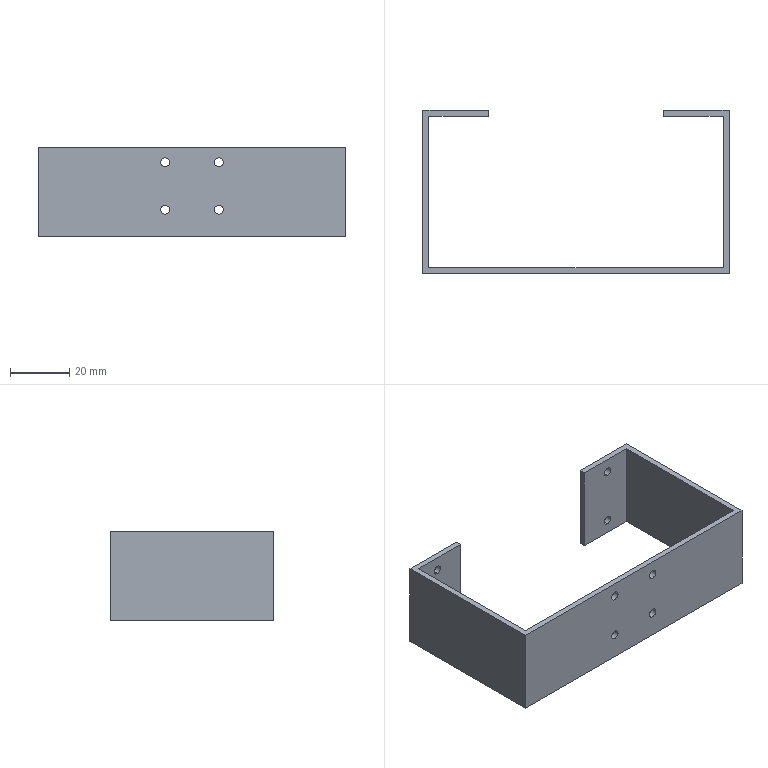Part | SolidWorks | features BaseBody 1 | 1 solid | 30 faces | box 103 x 55 x 30 mm | volume 14827 mm3 | cylinder 16 | plane 14 | commonest cylinder face diameters 3 x16
STEP:
#1=CARTESIAN_POINT('',(-11.413,0.,25.));
#2=VERTEX_POINT('',#1);
#3=CARTESIAN_POINT('',(-8.413,0.,25.));
#4=VERTEX_POINT('',#3);
#5=CARTESIAN_POINT('',(-9.913,0.,25.));
#6=DIRECTION('',(0.,-1.,0.));
#7=DIRECTION('',(1.,0.,0.));
#8=AXIS2_PLACEMENT_3D('',#5,#6,#7);
#9=CIRCLE('',#8,1.5);
#10=EDGE_CURVE('',#2,#4,#9,.T.);
#11=ORIENTED_EDGE('',*,*,#10,.F.);
#12=CARTESIAN_POINT('',(-11.413,-2.,25.));
#13=VERTEX_POINT('',#12);
#14=CARTESIAN_POINT('',(-11.413,8.,25.));
#15=DIRECTION('',(0.,-1.,0.));
#16=VECTOR('',#15,1000.);
#17=LINE('',#14,#16);
#18=EDGE_CURVE('',#2,#13,#17,.T.);
#19=ORIENTED_EDGE('',*,*,#18,.T.);
#20=CARTESIAN_POINT('',(-8.413,-2.,25.));
#21=VERTEX_POINT('',#20);
#22=CARTESIAN_POINT('',(-9.913,-2.,25.));
#23=DIRECTION('',(0.,1.,0.));
#24=DIRECTION('',(1.,0.,0.));
#25=AXIS2_PLACEMENT_3D('',#22,#23,#24);
#26=CIRCLE('',#25,1.5);
#27=EDGE_CURVE('',#21,#13,#26,.T.);
#28=ORIENTED_EDGE('',*,*,#27,.F.);
#29=CARTESIAN_POINT('',(-8.413,8.,25.));
#30=DIRECTION('',(0.,-1.,0.));
#31=VECTOR('',#30,1000.);
#32=LINE('',#29,#31);
#33=EDGE_CURVE('',#4,#21,#32,.T.);
#34=ORIENTED_EDGE('',*,*,#33,.F.);
#35=EDGE_LOOP('',(#11,#19,#28,#34));
#36=FACE_OUTER_BOUND('',#35,.T.);
#37=CARTESIAN_POINT('',(-9.913,8.,25.));
#38=DIRECTION('',(0.,-1.,0.));
#39=DIRECTION('',(1.,0.,0.));
#40=AXIS2_PLACEMENT_3D('',#37,#38,#39);
#41=CYLINDRICAL_SURFACE('',#40,1.5);
#42=ADVANCED_FACE('',(#36),#41,.F.);
#43=CARTESIAN_POINT('',(6.587,0.,9.));
#44=VERTEX_POINT('',#43);
#45=CARTESIAN_POINT('',(9.587,0.,9.));
#46=VERTEX_POINT('',#45);
#47=CARTESIAN_POINT('',(8.087,0.,9.));
#48=DIRECTION('',(0.,-1.,0.));
#49=DIRECTION('',(1.,0.,0.));
#50=AXIS2_PLACEMENT_3D('',#47,#48,#49);
#51=CIRCLE('',#50,1.5);
#52=EDGE_CURVE('',#44,#46,#51,.T.);
#53=ORIENTED_EDGE('',*,*,#52,.F.);
#54=CARTESIAN_POINT('',(6.587,-2.,9.));
#55=VERTEX_POINT('',#54);
#56=CARTESIAN_POINT('',(6.587,8.,9.));
#57=DIRECTION('',(0.,-1.,0.));
#58=VECTOR('',#57,1000.);
#59=LINE('',#56,#58);
#60=EDGE_CURVE('',#44,#55,#59,.T.);
#61=ORIENTED_EDGE('',*,*,#60,.T.);
#62=CARTESIAN_POINT('',(9.587,-2.,9.));
#63=VERTEX_POINT('',#62);
#64=CARTESIAN_POINT('',(8.087,-2.,9.));
#65=DIRECTION('',(0.,1.,0.));
#66=DIRECTION('',(1.,0.,0.));
#67=AXIS2_PLACEMENT_3D('',#64,#65,#66);
#68=CIRCLE('',#67,1.5);
#69=EDGE_CURVE('',#63,#55,#68,.T.);
#70=ORIENTED_EDGE('',*,*,#69,.F.);
#71=CARTESIAN_POINT('',(9.587,8.,9.));
#72=DIRECTION('',(0.,-1.,0.));
#73=VECTOR('',#72,1000.);
#74=LINE('',#71,#73);
#75=EDGE_CURVE('',#46,#63,#74,.T.);
#76=ORIENTED_EDGE('',*,*,#75,.F.);
#77=EDGE_LOOP('',(#53,#61,#70,#76));
#78=FACE_OUTER_BOUND('',#77,.T.);
#79=CARTESIAN_POINT('',(8.087,8.,9.));
#80=DIRECTION('',(0.,-1.,0.));
#81=DIRECTION('',(1.,0.,0.));
#82=AXIS2_PLACEMENT_3D('',#79,#80,#81);
#83=CYLINDRICAL_SURFACE('',#82,1.5);
#84=ADVANCED_FACE('',(#78),#83,.F.);
#85=CARTESIAN_POINT('',(-11.413,0.,9.));
#86=VERTEX_POINT('',#85);
#87=CARTESIAN_POINT('',(-8.413,0.,9.));
#88=VERTEX_POINT('',#87);
#89=CARTESIAN_POINT('',(-9.913,0.,9.));
#90=DIRECTION('',(0.,-1.,0.));
#91=DIRECTION('',(1.,0.,0.));
#92=AXIS2_PLACEMENT_3D('',#89,#90,#91);
#93=CIRCLE('',#92,1.5);
#94=EDGE_CURVE('',#86,#88,#93,.T.);
#95=ORIENTED_EDGE('',*,*,#94,.F.);
#96=CARTESIAN_POINT('',(-11.413,-2.,9.));
#97=VERTEX_POINT('',#96);
#98=CARTESIAN_POINT('',(-11.413,8.,9.));
#99=DIRECTION('',(0.,-1.,0.));
#100=VECTOR('',#99,1000.);
#101=LINE('',#98,#100);
#102=EDGE_CURVE('',#86,#97,#101,.T.);
#103=ORIENTED_EDGE('',*,*,#102,.T.);
#104=CARTESIAN_POINT('',(-8.413,-2.,9.));
#105=VERTEX_POINT('',#104);
#106=CARTESIAN_POINT('',(-9.913,-2.,9.));
#107=DIRECTION('',(0.,1.,0.));
#108=DIRECTION('',(1.,0.,0.));
#109=AXIS2_PLACEMENT_3D('',#106,#107,#108);
#110=CIRCLE('',#109,1.5);
#111=EDGE_CURVE('',#105,#97,#110,.T.);
#112=ORIENTED_EDGE('',*,*,#111,.F.);
#113=CARTESIAN_POINT('',(-8.413,8.,9.));
#114=DIRECTION('',(0.,-1.,0.));
#115=VECTOR('',#114,1000.);
#116=LINE('',#113,#115);
#117=EDGE_CURVE('',#88,#105,#116,.T.);
#118=ORIENTED_EDGE('',*,*,#117,.F.);
#119=EDGE_LOOP('',(#95,#103,#112,#118));
#120=FACE_OUTER_BOUND('',#119,.T.);
#121=CARTESIAN_POINT('',(-9.913,8.,9.));
#122=DIRECTION('',(0.,-1.,0.));
#123=DIRECTION('',(1.,0.,0.));
#124=AXIS2_PLACEMENT_3D('',#121,#122,#123);
#125=CYLINDRICAL_SURFACE('',#124,1.5);
#126=ADVANCED_FACE('',(#120),#125,.F.);
#127=CARTESIAN_POINT('',(6.587,0.,25.));
#128=VERTEX_POINT('',#127);
#129=CARTESIAN_POINT('',(9.587,0.,25.));
#130=VERTEX_POINT('',#129);
#131=CARTESIAN_POINT('',(8.087,0.,25.));
#132=DIRECTION('',(0.,-1.,0.));
#133=DIRECTION('',(1.,0.,0.));
#134=AXIS2_PLACEMENT_3D('',#131,#132,#133);
#135=CIRCLE('',#134,1.5);
#136=EDGE_CURVE('',#128,#130,#135,.T.);
#137=ORIENTED_EDGE('',*,*,#136,.F.);
#138=CARTESIAN_POINT('',(6.587,-2.,25.));
#139=VERTEX_POINT('',#138);
#140=CARTESIAN_POINT('',(6.587,8.,25.));
#141=DIRECTION('',(0.,-1.,0.));
#142=VECTOR('',#141,1000.);
#143=LINE('',#140,#142);
#144=EDGE_CURVE('',#128,#139,#143,.T.);
#145=ORIENTED_EDGE('',*,*,#144,.T.);
#146=CARTESIAN_POINT('',(9.587,-2.,25.));
#147=VERTEX_POINT('',#146);
#148=CARTESIAN_POINT('',(8.087,-2.,25.));
#149=DIRECTION('',(0.,1.,0.));
#150=DIRECTION('',(1.,0.,0.));
#151=AXIS2_PLACEMENT_3D('',#148,#149,#150);
#152=CIRCLE('',#151,1.5);
#153=EDGE_CURVE('',#147,#139,#152,.T.);
#154=ORIENTED_EDGE('',*,*,#153,.F.);
#155=CARTESIAN_POINT('',(9.587,8.,25.));
#156=DIRECTION('',(0.,-1.,0.));
#157=VECTOR('',#156,1000.);
#158=LINE('',#155,#157);
#159=EDGE_CURVE('',#130,#147,#158,.T.);
#160=ORIENTED_EDGE('',*,*,#159,.F.);
#161=EDGE_LOOP('',(#137,#145,#154,#160));
#162=FACE_OUTER_BOUND('',#161,.T.);
#163=CARTESIAN_POINT('',(8.087,8.,25.));
#164=DIRECTION('',(0.,-1.,0.));
#165=DIRECTION('',(1.,0.,0.));
#166=AXIS2_PLACEMENT_3D('',#163,#164,#165);
#167=CYLINDRICAL_SURFACE('',#166,1.5);
#168=ADVANCED_FACE('',(#162),#167,.F.);
#169=CARTESIAN_POINT('',(-41.413,51.,3.5));
#170=VERTEX_POINT('',#169);
#171=CARTESIAN_POINT('',(-41.413,51.,6.5));
#172=VERTEX_POINT('',#171);
#173=CARTESIAN_POINT('',(-41.413,51.,5.));
#174=DIRECTION('',(0.,1.,0.));
#175=DIRECTION('',(0.,0.,1.));
#176=AXIS2_PLACEMENT_3D('',#173,#174,#175);
#177=CIRCLE('',#176,1.5);
#178=EDGE_CURVE('',#170,#172,#177,.T.);
#179=ORIENTED_EDGE('',*,*,#178,.F.);
#180=CARTESIAN_POINT('',(-41.413,53.,3.5));
#181=VERTEX_POINT('',#180);
#182=CARTESIAN_POINT('',(-41.413,48.,3.5));
#183=DIRECTION('',(0.,1.,0.));
#184=VECTOR('',#183,1000.);
#185=LINE('',#182,#184);
#186=EDGE_CURVE('',#170,#181,#185,.T.);
#187=ORIENTED_EDGE('',*,*,#186,.T.);
#188=CARTESIAN_POINT('',(-41.413,53.,6.5));
#189=VERTEX_POINT('',#188);
#190=CARTESIAN_POINT('',(-41.413,53.,5.));
#191=DIRECTION('',(0.,-1.,0.));
#192=DIRECTION('',(0.,0.,1.));
#193=AXIS2_PLACEMENT_3D('',#190,#191,#192);
#194=CIRCLE('',#193,1.5);
#195=EDGE_CURVE('',#189,#181,#194,.T.);
#196=ORIENTED_EDGE('',*,*,#195,.F.);
#197=CARTESIAN_POINT('',(-41.413,48.,6.5));
#198=DIRECTION('',(0.,1.,0.));
#199=VECTOR('',#198,1000.);
#200=LINE('',#197,#199);
#201=EDGE_CURVE('',#172,#189,#200,.T.);
#202=ORIENTED_EDGE('',*,*,#201,.F.);
#203=EDGE_LOOP('',(#179,#187,#196,#202));
#204=FACE_OUTER_BOUND('',#203,.T.);
#205=CARTESIAN_POINT('',(-41.413,48.,5.));
#206=DIRECTION('',(0.,1.,0.));
#207=DIRECTION('',(0.,0.,1.));
#208=AXIS2_PLACEMENT_3D('',#205,#206,#207);
#209=CYLINDRICAL_SURFACE('',#208,1.5);
#210=ADVANCED_FACE('',(#204),#209,.F.);
#211=CARTESIAN_POINT('',(-41.413,51.,23.5));
#212=VERTEX_POINT('',#211);
#213=CARTESIAN_POINT('',(-41.413,51.,26.5));
#214=VERTEX_POINT('',#213);
#215=CARTESIAN_POINT('',(-41.413,51.,25.));
#216=DIRECTION('',(0.,1.,0.));
#217=DIRECTION('',(0.,0.,1.));
#218=AXIS2_PLACEMENT_3D('',#215,#216,#217);
#219=CIRCLE('',#218,1.5);
#220=EDGE_CURVE('',#212,#214,#219,.T.);
#221=ORIENTED_EDGE('',*,*,#220,.F.);
#222=CARTESIAN_POINT('',(-41.413,53.,23.5));
#223=VERTEX_POINT('',#222);
#224=CARTESIAN_POINT('',(-41.413,48.,23.5));
#225=DIRECTION('',(0.,1.,0.));
#226=VECTOR('',#225,1000.);
#227=LINE('',#224,#226);
#228=EDGE_CURVE('',#212,#223,#227,.T.);
#229=ORIENTED_EDGE('',*,*,#228,.T.);
#230=CARTESIAN_POINT('',(-41.413,53.,26.5));
#231=VERTEX_POINT('',#230);
#232=CARTESIAN_POINT('',(-41.413,53.,25.));
#233=DIRECTION('',(0.,-1.,0.));
#234=DIRECTION('',(0.,0.,1.));
#235=AXIS2_PLACEMENT_3D('',#232,#233,#234);
#236=CIRCLE('',#235,1.5);
#237=EDGE_CURVE('',#231,#223,#236,.T.);
#238=ORIENTED_EDGE('',*,*,#237,.F.);
#239=CARTESIAN_POINT('',(-41.413,48.,26.5));
#240=DIRECTION('',(0.,1.,0.));
#241=VECTOR('',#240,1000.);
#242=LINE('',#239,#241);
#243=EDGE_CURVE('',#214,#231,#242,.T.);
#244=ORIENTED_EDGE('',*,*,#243,.F.);
#245=EDGE_LOOP('',(#221,#229,#238,#244));
#246=FACE_OUTER_BOUND('',#245,.T.);
#247=CARTESIAN_POINT('',(-41.413,48.,25.));
#248=DIRECTION('',(0.,1.,0.));
#249=DIRECTION('',(0.,0.,1.));
#250=AXIS2_PLACEMENT_3D('',#247,#248,#249);
#251=CYLINDRICAL_SURFACE('',#250,1.5);
#252=ADVANCED_FACE('',(#246),#251,.F.);
#253=CARTESIAN_POINT('',(39.587,51.,26.5));
#254=VERTEX_POINT('',#253);
#255=CARTESIAN_POINT('',(39.587,51.,23.5));
#256=VERTEX_POINT('',#255);
#257=CARTESIAN_POINT('',(39.587,51.,25.));
#258=DIRECTION('',(0.,-1.,0.));
#259=DIRECTION('',(0.,0.,1.));
#260=AXIS2_PLACEMENT_3D('',#257,#258,#259);
#261=CIRCLE('',#260,1.5);
#262=EDGE_CURVE('',#254,#256,#261,.T.);
#263=ORIENTED_EDGE('',*,*,#262,.T.);
#264=CARTESIAN_POINT('',(39.587,53.,23.5));
#265=VERTEX_POINT('',#264);
#266=CARTESIAN_POINT('',(39.587,48.,23.5));
#267=DIRECTION('',(0.,1.,0.));
#268=VECTOR('',#267,1000.);
#269=LINE('',#266,#268);
#270=EDGE_CURVE('',#256,#265,#269,.T.);
#271=ORIENTED_EDGE('',*,*,#270,.T.);
#272=CARTESIAN_POINT('',(39.587,53.,26.5));
#273=VERTEX_POINT('',#272);
#274=CARTESIAN_POINT('',(39.587,53.,25.));
#275=DIRECTION('',(0.,1.,0.));
#276=DIRECTION('',(0.,0.,1.));
#277=AXIS2_PLACEMENT_3D('',#274,#275,#276);
#278=CIRCLE('',#277,1.5);
#279=EDGE_CURVE('',#265,#273,#278,.T.);
#280=ORIENTED_EDGE('',*,*,#279,.T.);
#281=CARTESIAN_POINT('',(39.587,48.,26.5));
#282=DIRECTION('',(0.,1.,0.));
#283=VECTOR('',#282,1000.);
#284=LINE('',#281,#283);
#285=EDGE_CURVE('',#254,#273,#284,.T.);
#286=ORIENTED_EDGE('',*,*,#285,.F.);
#287=EDGE_LOOP('',(#263,#271,#280,#286));
#288=FACE_OUTER_BOUND('',#287,.T.);
#289=CARTESIAN_POINT('',(39.587,48.,25.));
#290=DIRECTION('',(0.,1.,0.));
#291=DIRECTION('',(0.,0.,1.));
#292=AXIS2_PLACEMENT_3D('',#289,#290,#291);
#293=CYLINDRICAL_SURFACE('',#292,1.5);
#294=ADVANCED_FACE('',(#288),#293,.F.);
#295=CARTESIAN_POINT('',(39.587,51.,6.5));
#296=VERTEX_POINT('',#295);
#297=CARTESIAN_POINT('',(39.587,51.,3.5));
#298=VERTEX_POINT('',#297);
#299=CARTESIAN_POINT('',(39.587,51.,5.));
#300=DIRECTION('',(0.,-1.,0.));
#301=DIRECTION('',(0.,0.,1.));
#302=AXIS2_PLACEMENT_3D('',#299,#300,#301);
#303=CIRCLE('',#302,1.5);
#304=EDGE_CURVE('',#296,#298,#303,.T.);
#305=ORIENTED_EDGE('',*,*,#304,.T.);
#306=CARTESIAN_POINT('',(39.587,53.,3.5));
#307=VERTEX_POINT('',#306);
#308=CARTESIAN_POINT('',(39.587,48.,3.5));
#309=DIRECTION('',(0.,1.,0.));
#310=VECTOR('',#309,1000.);
#311=LINE('',#308,#310);
#312=EDGE_CURVE('',#298,#307,#311,.T.);
#313=ORIENTED_EDGE('',*,*,#312,.T.);
#314=CARTESIAN_POINT('',(39.587,53.,6.5));
#315=VERTEX_POINT('',#314);
#316=CARTESIAN_POINT('',(39.587,53.,5.));
#317=DIRECTION('',(0.,1.,0.));
#318=DIRECTION('',(0.,0.,1.));
#319=AXIS2_PLACEMENT_3D('',#316,#317,#318);
#320=CIRCLE('',#319,1.5);
#321=EDGE_CURVE('',#307,#315,#320,.T.);
#322=ORIENTED_EDGE('',*,*,#321,.T.);
#323=CARTESIAN_POINT('',(39.587,48.,6.5));
#324=DIRECTION('',(0.,1.,0.));
#325=VECTOR('',#324,1000.);
#326=LINE('',#323,#325);
#327=EDGE_CURVE('',#296,#315,#326,.T.);
#328=ORIENTED_EDGE('',*,*,#327,.F.);
#329=EDGE_LOOP('',(#305,#313,#322,#328));
#330=FACE_OUTER_BOUND('',#329,.T.);
#331=CARTESIAN_POINT('',(39.587,48.,5.));
#332=DIRECTION('',(0.,1.,0.));
#333=DIRECTION('',(0.,0.,1.));
#334=AXIS2_PLACEMENT_3D('',#331,#332,#333);
#335=CYLINDRICAL_SURFACE('',#334,1.5);
#336=ADVANCED_FACE('',(#330),#335,.F.);
#337=CARTESIAN_POINT('',(50.587,-2.,30.));
#338=VERTEX_POINT('',#337);
#339=CARTESIAN_POINT('',(-52.413,-2.,30.));
#340=VERTEX_POINT('',#339);
#341=CARTESIAN_POINT('',(0.,-2.,30.));
#342=DIRECTION('',(-1.,0.,0.));
#343=VECTOR('',#342,1000.);
#344=LINE('',#341,#343);
#345=EDGE_CURVE('',#338,#340,#344,.T.);
#346=ORIENTED_EDGE('',*,*,#345,.T.);
#347=CARTESIAN_POINT('',(-52.413,-2.,0.));
#348=VERTEX_POINT('',#347);
#349=CARTESIAN_POINT('',(-52.413,-2.,30.));
#350=DIRECTION('',(0.,0.,-1.));
#351=VECTOR('',#350,1000.);
#352=LINE('',#349,#351);
#353=EDGE_CURVE('',#340,#348,#352,.T.);
#354=ORIENTED_EDGE('',*,*,#353,.T.);
#355=CARTESIAN_POINT('',(50.587,-2.,0.));
#356=VERTEX_POINT('',#355);
#357=CARTESIAN_POINT('',(0.,-2.,0.));
#358=DIRECTION('',(1.,0.,0.));
#359=VECTOR('',#358,1000.);
#360=LINE('',#357,#359);
#361=EDGE_CURVE('',#348,#356,#360,.T.);
#362=ORIENTED_EDGE('',*,*,#361,.T.);
#363=CARTESIAN_POINT('',(50.587,-2.,30.));
#364=DIRECTION('',(0.,0.,1.));
#365=VECTOR('',#364,1000.);
#366=LINE('',#363,#365);
#367=EDGE_CURVE('',#356,#338,#366,.T.);
#368=ORIENTED_EDGE('',*,*,#367,.T.);
#369=EDGE_LOOP('',(#346,#354,#362,#368));
#370=FACE_OUTER_BOUND('',#369,.T.);
#371=ORIENTED_EDGE('',*,*,#27,.T.);
#372=CARTESIAN_POINT('',(-9.913,-2.,25.));
#373=DIRECTION('',(0.,1.,0.));
#374=DIRECTION('',(1.,0.,0.));
#375=AXIS2_PLACEMENT_3D('',#372,#373,#374);
#376=CIRCLE('',#375,1.5);
#377=EDGE_CURVE('',#13,#21,#376,.T.);
#378=ORIENTED_EDGE('',*,*,#377,.T.);
#379=EDGE_LOOP('',(#371,#378));
#380=FACE_BOUND('',#379,.T.);
#381=ORIENTED_EDGE('',*,*,#69,.T.);
#382=CARTESIAN_POINT('',(8.087,-2.,9.));
#383=DIRECTION('',(0.,1.,0.));
#384=DIRECTION('',(1.,0.,0.));
#385=AXIS2_PLACEMENT_3D('',#382,#383,#384);
#386=CIRCLE('',#385,1.5);
#387=EDGE_CURVE('',#55,#63,#386,.T.);
#388=ORIENTED_EDGE('',*,*,#387,.T.);
#389=EDGE_LOOP('',(#381,#388));
#390=FACE_BOUND('',#389,.T.);
#391=ORIENTED_EDGE('',*,*,#111,.T.);
#392=CARTESIAN_POINT('',(-9.913,-2.,9.));
#393=DIRECTION('',(0.,1.,0.));
#394=DIRECTION('',(1.,0.,0.));
#395=AXIS2_PLACEMENT_3D('',#392,#393,#394);
#396=CIRCLE('',#395,1.5);
#397=EDGE_CURVE('',#97,#105,#396,.T.);
#398=ORIENTED_EDGE('',*,*,#397,.T.);
#399=EDGE_LOOP('',(#391,#398));
#400=FACE_BOUND('',#399,.T.);
#401=ORIENTED_EDGE('',*,*,#153,.T.);
#402=CARTESIAN_POINT('',(8.087,-2.,25.));
#403=DIRECTION('',(0.,1.,0.));
#404=DIRECTION('',(1.,0.,0.));
#405=AXIS2_PLACEMENT_3D('',#402,#403,#404);
#406=CIRCLE('',#405,1.5);
#407=EDGE_CURVE('',#139,#147,#406,.T.);
#408=ORIENTED_EDGE('',*,*,#407,.T.);
#409=EDGE_LOOP('',(#401,#408));
#410=FACE_BOUND('',#409,.T.);
#411=CARTESIAN_POINT('',(0.,-2.,30.));
#412=DIRECTION('',(0.,-1.,0.));
#413=DIRECTION('',(1.,0.,0.));
#414=AXIS2_PLACEMENT_3D('',#411,#412,#413);
#415=PLANE('',#414);
#416=ADVANCED_FACE('',(#370,#380,#390,#400,#410),#415,.T.);
#417=CARTESIAN_POINT('',(-52.413,53.,30.));
#418=VERTEX_POINT('',#417);
#419=CARTESIAN_POINT('',(-52.413,0.,30.));
#420=DIRECTION('',(0.,1.,0.));
#421=VECTOR('',#420,1000.);
#422=LINE('',#419,#421);
#423=EDGE_CURVE('',#340,#418,#422,.T.);
#424=ORIENTED_EDGE('',*,*,#423,.T.);
#425=CARTESIAN_POINT('',(-52.413,53.,0.));
#426=VERTEX_POINT('',#425);
#427=CARTESIAN_POINT('',(-52.413,53.,30.));
#428=DIRECTION('',(0.,0.,-1.));
#429=VECTOR('',#428,1000.);
#430=LINE('',#427,#429);
#431=EDGE_CURVE('',#418,#426,#430,.T.);
#432=ORIENTED_EDGE('',*,*,#431,.T.);
#433=CARTESIAN_POINT('',(-52.413,0.,0.));
#434=DIRECTION('',(0.,-1.,0.));
#435=VECTOR('',#434,1000.);
#436=LINE('',#433,#435);
#437=EDGE_CURVE('',#426,#348,#436,.T.);
#438=ORIENTED_EDGE('',*,*,#437,.T.);
#439=ORIENTED_EDGE('',*,*,#353,.F.);
#440=EDGE_LOOP('',(#424,#432,#438,#439));
#441=FACE_OUTER_BOUND('',#440,.T.);
#442=CARTESIAN_POINT('',(-52.413,0.,30.));
#443=DIRECTION('',(-1.,0.,0.));
#444=DIRECTION('',(0.,0.,1.));
#445=AXIS2_PLACEMENT_3D('',#442,#443,#444);
#446=PLANE('',#445);
#447=ADVANCED_FACE('',(#441),#446,.T.);
#448=CARTESIAN_POINT('',(-30.413,53.,30.));
#449=VERTEX_POINT('',#448);
#450=CARTESIAN_POINT('',(0.,53.,30.));
#451=DIRECTION('',(-1.,0.,0.));
#452=VECTOR('',#451,1000.);
#453=LINE('',#450,#452);
#454=EDGE_CURVE('',#449,#418,#453,.T.);
#455=ORIENTED_EDGE('',*,*,#454,.T.);
#456=ORIENTED_EDGE('',*,*,#423,.F.);
#457=ORIENTED_EDGE('',*,*,#345,.F.);
#458=CARTESIAN_POINT('',(50.587,53.,30.));
#459=VERTEX_POINT('',#458);
#460=CARTESIAN_POINT('',(50.587,0.,30.));
#461=DIRECTION('',(0.,1.,0.));
#462=VECTOR('',#461,1000.);
#463=LINE('',#460,#462);
#464=EDGE_CURVE('',#338,#459,#463,.T.);
#465=ORIENTED_EDGE('',*,*,#464,.T.);
#466=CARTESIAN_POINT('',(28.587,53.,30.));
#467=VERTEX_POINT('',#466);
#468=CARTESIAN_POINT('',(0.,53.,30.));
#469=DIRECTION('',(-1.,0.,0.));
#470=VECTOR('',#469,1000.);
#471=LINE('',#468,#470);
#472=EDGE_CURVE('',#459,#467,#471,.T.);
#473=ORIENTED_EDGE('',*,*,#472,.T.);
#474=CARTESIAN_POINT('',(28.587,51.,30.));
#475=VERTEX_POINT('',#474);
#476=CARTESIAN_POINT('',(28.587,0.,30.));
#477=DIRECTION('',(0.,-1.,0.));
#478=VECTOR('',#477,1000.);
#479=LINE('',#476,#478);
#480=EDGE_CURVE('',#467,#475,#479,.T.);
#481=ORIENTED_EDGE('',*,*,#480,.T.);
#482=CARTESIAN_POINT('',(48.587,51.,30.));
#483=VERTEX_POINT('',#482);
#484=CARTESIAN_POINT('',(0.,51.,30.));
#485=DIRECTION('',(1.,0.,0.));
#486=VECTOR('',#485,1000.);
#487=LINE('',#484,#486);
#488=EDGE_CURVE('',#475,#483,#487,.T.);
#489=ORIENTED_EDGE('',*,*,#488,.T.);
#490=CARTESIAN_POINT('',(48.587,0.,30.));
#491=VERTEX_POINT('',#490);
#492=CARTESIAN_POINT('',(48.587,0.,30.));
#493=DIRECTION('',(0.,-1.,0.));
#494=VECTOR('',#493,1000.);
#495=LINE('',#492,#494);
#496=EDGE_CURVE('',#483,#491,#495,.T.);
#497=ORIENTED_EDGE('',*,*,#496,.T.);
#498=CARTESIAN_POINT('',(-50.413,0.,30.));
#499=VERTEX_POINT('',#498);
#500=CARTESIAN_POINT('',(0.,0.,30.));
#501=DIRECTION('',(-1.,0.,0.));
#502=VECTOR('',#501,1000.);
#503=LINE('',#500,#502);
#504=EDGE_CURVE('',#491,#499,#503,.T.);
#505=ORIENTED_EDGE('',*,*,#504,.T.);
#506=CARTESIAN_POINT('',(-50.413,51.,30.));
#507=VERTEX_POINT('',#506);
#508=CARTESIAN_POINT('',(-50.413,0.,30.));
#509=DIRECTION('',(0.,1.,0.));
#510=VECTOR('',#509,1000.);
#511=LINE('',#508,#510);
#512=EDGE_CURVE('',#499,#507,#511,.T.);
#513=ORIENTED_EDGE('',*,*,#512,.T.);
#514=CARTESIAN_POINT('',(-30.413,51.,30.));
#515=VERTEX_POINT('',#514);
#516=CARTESIAN_POINT('',(0.,51.,30.));
#517=DIRECTION('',(1.,0.,0.));
#518=VECTOR('',#517,1000.);
#519=LINE('',#516,#518);
#520=EDGE_CURVE('',#507,#515,#519,.T.);
#521=ORIENTED_EDGE('',*,*,#520,.T.);
#522=CARTESIAN_POINT('',(-30.413,0.,30.));
#523=DIRECTION('',(0.,1.,0.));
#524=VECTOR('',#523,1000.);
#525=LINE('',#522,#524);
#526=EDGE_CURVE('',#515,#449,#525,.T.);
#527=ORIENTED_EDGE('',*,*,#526,.T.);
#528=EDGE_LOOP('',(#455,#456,#457,#465,#473,#481,#489,#497,#505,#513,#521,#527));
#529=FACE_OUTER_BOUND('',#528,.T.);
#530=CARTESIAN_POINT('',(0.,0.,30.));
#531=DIRECTION('',(0.,0.,1.));
#532=DIRECTION('',(1.,0.,0.));
#533=AXIS2_PLACEMENT_3D('',#530,#531,#532);
#534=PLANE('',#533);
#535=ADVANCED_FACE('',(#529),#534,.T.);
#536=CARTESIAN_POINT('',(50.587,53.,0.));
#537=VERTEX_POINT('',#536);
#538=CARTESIAN_POINT('',(50.587,53.,30.));
#539=DIRECTION('',(0.,0.,-1.));
#540=VECTOR('',#539,1000.);
#541=LINE('',#538,#540);
#542=EDGE_CURVE('',#459,#537,#541,.T.);
#543=ORIENTED_EDGE('',*,*,#542,.F.);
#544=ORIENTED_EDGE('',*,*,#464,.F.);
#545=ORIENTED_EDGE('',*,*,#367,.F.);
#546=CARTESIAN_POINT('',(50.587,0.,0.));
#547=DIRECTION('',(0.,-1.,0.));
#548=VECTOR('',#547,1000.);
#549=LINE('',#546,#548);
#550=EDGE_CURVE('',#537,#356,#549,.T.);
#551=ORIENTED_EDGE('',*,*,#550,.F.);
#552=EDGE_LOOP('',(#543,#544,#545,#551));
#553=FACE_OUTER_BOUND('',#552,.T.);
#554=CARTESIAN_POINT('',(50.587,0.,30.));
#555=DIRECTION('',(-1.,0.,0.));
#556=DIRECTION('',(0.,-1.,0.));
#557=AXIS2_PLACEMENT_3D('',#554,#555,#556);
#558=PLANE('',#557);
#559=ADVANCED_FACE('',(#553),#558,.F.);
#560=ORIENTED_EDGE('',*,*,#437,.F.);
#561=CARTESIAN_POINT('',(-30.413,53.,0.));
#562=VERTEX_POINT('',#561);
#563=CARTESIAN_POINT('',(0.,53.,0.));
#564=DIRECTION('',(-1.,0.,0.));
#565=VECTOR('',#564,1000.);
#566=LINE('',#563,#565);
#567=EDGE_CURVE('',#562,#426,#566,.T.);
#568=ORIENTED_EDGE('',*,*,#567,.F.);
#569=CARTESIAN_POINT('',(-30.413,51.,0.));
#570=VERTEX_POINT('',#569);
#571=CARTESIAN_POINT('',(-30.413,0.,0.));
#572=DIRECTION('',(0.,1.,0.));
#573=VECTOR('',#572,1000.);
#574=LINE('',#571,#573);
#575=EDGE_CURVE('',#570,#562,#574,.T.);
#576=ORIENTED_EDGE('',*,*,#575,.F.);
#577=CARTESIAN_POINT('',(-50.413,51.,0.));
#578=VERTEX_POINT('',#577);
#579=CARTESIAN_POINT('',(0.,51.,0.));
#580=DIRECTION('',(1.,0.,0.));
#581=VECTOR('',#580,1000.);
#582=LINE('',#579,#581);
#583=EDGE_CURVE('',#578,#570,#582,.T.);
#584=ORIENTED_EDGE('',*,*,#583,.F.);
#585=CARTESIAN_POINT('',(-50.413,0.,0.));
#586=VERTEX_POINT('',#585);
#587=CARTESIAN_POINT('',(-50.413,0.,0.));
#588=DIRECTION('',(0.,1.,0.));
#589=VECTOR('',#588,1000.);
#590=LINE('',#587,#589);
#591=EDGE_CURVE('',#586,#578,#590,.T.);
#592=ORIENTED_EDGE('',*,*,#591,.F.);
#593=CARTESIAN_POINT('',(48.587,0.,0.));
#594=VERTEX_POINT('',#593);
#595=CARTESIAN_POINT('',(0.,0.,0.));
#596=DIRECTION('',(-1.,0.,0.));
#597=VECTOR('',#596,1000.);
#598=LINE('',#595,#597);
#599=EDGE_CURVE('',#594,#586,#598,.T.);
#600=ORIENTED_EDGE('',*,*,#599,.F.);
#601=CARTESIAN_POINT('',(48.587,51.,0.));
#602=VERTEX_POINT('',#601);
#603=CARTESIAN_POINT('',(48.587,0.,0.));
#604=DIRECTION('',(0.,-1.,0.));
#605=VECTOR('',#604,1000.);
#606=LINE('',#603,#605);
#607=EDGE_CURVE('',#602,#594,#606,.T.);
#608=ORIENTED_EDGE('',*,*,#607,.F.);
#609=CARTESIAN_POINT('',(28.587,51.,0.));
#610=VERTEX_POINT('',#609);
#611=CARTESIAN_POINT('',(0.,51.,0.));
#612=DIRECTION('',(1.,0.,0.));
#613=VECTOR('',#612,1000.);
#614=LINE('',#611,#613);
#615=EDGE_CURVE('',#610,#602,#614,.T.);
#616=ORIENTED_EDGE('',*,*,#615,.F.);
#617=CARTESIAN_POINT('',(28.587,53.,0.));
#618=VERTEX_POINT('',#617);
#619=CARTESIAN_POINT('',(28.587,0.,0.));
#620=DIRECTION('',(0.,-1.,0.));
#621=VECTOR('',#620,1000.);
#622=LINE('',#619,#621);
#623=EDGE_CURVE('',#618,#610,#622,.T.);
#624=ORIENTED_EDGE('',*,*,#623,.F.);
#625=CARTESIAN_POINT('',(0.,53.,0.));
#626=DIRECTION('',(-1.,0.,0.));
#627=VECTOR('',#626,1000.);
#628=LINE('',#625,#627);
#629=EDGE_CURVE('',#537,#618,#628,.T.);
#630=ORIENTED_EDGE('',*,*,#629,.F.);
#631=ORIENTED_EDGE('',*,*,#550,.T.);
#632=ORIENTED_EDGE('',*,*,#361,.F.);
#633=EDGE_LOOP('',(#560,#568,#576,#584,#592,#600,#608,#616,#624,#630,#631,#632));
#634=FACE_OUTER_BOUND('',#633,.T.);
#635=CARTESIAN_POINT('',(0.,0.,0.));
#636=DIRECTION('',(0.,0.,1.));
#637=DIRECTION('',(1.,0.,0.));
#638=AXIS2_PLACEMENT_3D('',#635,#636,#637);
#639=PLANE('',#638);
#640=ADVANCED_FACE('',(#634),#639,.F.);
#641=ORIENTED_EDGE('',*,*,#18,.F.);
#642=CARTESIAN_POINT('',(-9.913,0.,25.));
#643=DIRECTION('',(0.,-1.,0.));
#644=DIRECTION('',(1.,0.,0.));
#645=AXIS2_PLACEMENT_3D('',#642,#643,#644);
#646=CIRCLE('',#645,1.5);
#647=EDGE_CURVE('',#4,#2,#646,.T.);
#648=ORIENTED_EDGE('',*,*,#647,.F.);
#649=ORIENTED_EDGE('',*,*,#33,.T.);
#650=ORIENTED_EDGE('',*,*,#377,.F.);
#651=EDGE_LOOP('',(#641,#648,#649,#650));
#652=FACE_OUTER_BOUND('',#651,.T.);
#653=CARTESIAN_POINT('',(-9.913,8.,25.));
#654=DIRECTION('',(0.,-1.,0.));
#655=DIRECTION('',(1.,0.,0.));
#656=AXIS2_PLACEMENT_3D('',#653,#654,#655);
#657=CYLINDRICAL_SURFACE('',#656,1.5);
#658=ADVANCED_FACE('',(#652),#657,.F.);
#659=ORIENTED_EDGE('',*,*,#60,.F.);
#660=CARTESIAN_POINT('',(8.087,0.,9.));
#661=DIRECTION('',(0.,-1.,0.));
#662=DIRECTION('',(1.,0.,0.));
#663=AXIS2_PLACEMENT_3D('',#660,#661,#662);
#664=CIRCLE('',#663,1.5);
#665=EDGE_CURVE('',#46,#44,#664,.T.);
#666=ORIENTED_EDGE('',*,*,#665,.F.);
#667=ORIENTED_EDGE('',*,*,#75,.T.);
#668=ORIENTED_EDGE('',*,*,#387,.F.);
#669=EDGE_LOOP('',(#659,#666,#667,#668));
#670=FACE_OUTER_BOUND('',#669,.T.);
#671=CARTESIAN_POINT('',(8.087,8.,9.));
#672=DIRECTION('',(0.,-1.,0.));
#673=DIRECTION('',(1.,0.,0.));
#674=AXIS2_PLACEMENT_3D('',#671,#672,#673);
#675=CYLINDRICAL_SURFACE('',#674,1.5);
#676=ADVANCED_FACE('',(#670),#675,.F.);
#677=ORIENTED_EDGE('',*,*,#102,.F.);
#678=CARTESIAN_POINT('',(-9.913,0.,9.));
#679=DIRECTION('',(0.,-1.,0.));
#680=DIRECTION('',(1.,0.,0.));
#681=AXIS2_PLACEMENT_3D('',#678,#679,#680);
#682=CIRCLE('',#681,1.5);
#683=EDGE_CURVE('',#88,#86,#682,.T.);
#684=ORIENTED_EDGE('',*,*,#683,.F.);
#685=ORIENTED_EDGE('',*,*,#117,.T.);
#686=ORIENTED_EDGE('',*,*,#397,.F.);
#687=EDGE_LOOP('',(#677,#684,#685,#686));
#688=FACE_OUTER_BOUND('',#687,.T.);
#689=CARTESIAN_POINT('',(-9.913,8.,9.));
#690=DIRECTION('',(0.,-1.,0.));
#691=DIRECTION('',(1.,0.,0.));
#692=AXIS2_PLACEMENT_3D('',#689,#690,#691);
#693=CYLINDRICAL_SURFACE('',#692,1.5);
#694=ADVANCED_FACE('',(#688),#693,.F.);
#695=ORIENTED_EDGE('',*,*,#144,.F.);
#696=CARTESIAN_POINT('',(8.087,0.,25.));
#697=DIRECTION('',(0.,-1.,0.));
#698=DIRECTION('',(1.,0.,0.));
#699=AXIS2_PLACEMENT_3D('',#696,#697,#698);
#700=CIRCLE('',#699,1.5);
#701=EDGE_CURVE('',#130,#128,#700,.T.);
#702=ORIENTED_EDGE('',*,*,#701,.F.);
#703=ORIENTED_EDGE('',*,*,#159,.T.);
#704=ORIENTED_EDGE('',*,*,#407,.F.);
#705=EDGE_LOOP('',(#695,#702,#703,#704));
#706=FACE_OUTER_BOUND('',#705,.T.);
#707=CARTESIAN_POINT('',(8.087,8.,25.));
#708=DIRECTION('',(0.,-1.,0.));
#709=DIRECTION('',(1.,0.,0.));
#710=AXIS2_PLACEMENT_3D('',#707,#708,#709);
#711=CYLINDRICAL_SURFACE('',#710,1.5);
#712=ADVANCED_FACE('',(#706),#711,.F.);
#713=ORIENTED_EDGE('',*,*,#454,.F.);
#714=CARTESIAN_POINT('',(-30.413,53.,30.));
#715=DIRECTION('',(0.,0.,-1.));
#716=VECTOR('',#715,1000.);
#717=LINE('',#714,#716);
#718=EDGE_CURVE('',#449,#562,#717,.T.);
#719=ORIENTED_EDGE('',*,*,#718,.T.);
#720=ORIENTED_EDGE('',*,*,#567,.T.);
#721=ORIENTED_EDGE('',*,*,#431,.F.);
#722=EDGE_LOOP('',(#713,#719,#720,#721));
#723=FACE_OUTER_BOUND('',#722,.T.);
#724=ORIENTED_EDGE('',*,*,#195,.T.);
#725=CARTESIAN_POINT('',(-41.413,53.,5.));
#726=DIRECTION('',(0.,-1.,0.));
#727=DIRECTION('',(0.,0.,1.));
#728=AXIS2_PLACEMENT_3D('',#725,#726,#727);
#729=CIRCLE('',#728,1.5);
#730=EDGE_CURVE('',#181,#189,#729,.T.);
#731=ORIENTED_EDGE('',*,*,#730,.T.);
#732=EDGE_LOOP('',(#724,#731));
#733=FACE_BOUND('',#732,.T.);
#734=ORIENTED_EDGE('',*,*,#237,.T.);
#735=CARTESIAN_POINT('',(-41.413,53.,25.));
#736=DIRECTION('',(0.,-1.,0.));
#737=DIRECTION('',(0.,0.,1.));
#738=AXIS2_PLACEMENT_3D('',#735,#736,#737);
#739=CIRCLE('',#738,1.5);
#740=EDGE_CURVE('',#223,#231,#739,.T.);
#741=ORIENTED_EDGE('',*,*,#740,.T.);
#742=EDGE_LOOP('',(#734,#741));
#743=FACE_BOUND('',#742,.T.);
#744=CARTESIAN_POINT('',(0.,53.,30.));
#745=DIRECTION('',(0.,1.,0.));
#746=DIRECTION('',(0.,0.,1.));
#747=AXIS2_PLACEMENT_3D('',#744,#745,#746);
#748=PLANE('',#747);
#749=ADVANCED_FACE('',(#723,#733,#743),#748,.T.);
#750=ORIENTED_EDGE('',*,*,#526,.F.);
#751=CARTESIAN_POINT('',(-30.413,51.,30.));
#752=DIRECTION('',(0.,0.,-1.));
#753=VECTOR('',#752,1000.);
#754=LINE('',#751,#753);
#755=EDGE_CURVE('',#515,#570,#754,.T.);
#756=ORIENTED_EDGE('',*,*,#755,.T.);
#757=ORIENTED_EDGE('',*,*,#575,.T.);
#758=ORIENTED_EDGE('',*,*,#718,.F.);
#759=EDGE_LOOP('',(#750,#756,#757,#758));
#760=FACE_OUTER_BOUND('',#759,.T.);
#761=CARTESIAN_POINT('',(-30.413,0.,30.));
#762=DIRECTION('',(1.,0.,0.));
#763=DIRECTION('',(0.,0.,-1.));
#764=AXIS2_PLACEMENT_3D('',#761,#762,#763);
#765=PLANE('',#764);
#766=ADVANCED_FACE('',(#760),#765,.T.);
#767=ORIENTED_EDGE('',*,*,#520,.F.);
#768=CARTESIAN_POINT('',(-50.413,51.,30.));
#769=DIRECTION('',(0.,0.,-1.));
#770=VECTOR('',#769,1000.);
#771=LINE('',#768,#770);
#772=EDGE_CURVE('',#507,#578,#771,.T.);
#773=ORIENTED_EDGE('',*,*,#772,.T.);
#774=ORIENTED_EDGE('',*,*,#583,.T.);
#775=ORIENTED_EDGE('',*,*,#755,.F.);
#776=EDGE_LOOP('',(#767,#773,#774,#775));
#777=FACE_OUTER_BOUND('',#776,.T.);
#778=CARTESIAN_POINT('',(-41.413,51.,5.));
#779=DIRECTION('',(0.,1.,0.));
#780=DIRECTION('',(0.,0.,1.));
#781=AXIS2_PLACEMENT_3D('',#778,#779,#780);
#782=CIRCLE('',#781,1.5);
#783=EDGE_CURVE('',#172,#170,#782,.T.);
#784=ORIENTED_EDGE('',*,*,#783,.T.);
#785=ORIENTED_EDGE('',*,*,#178,.T.);
#786=EDGE_LOOP('',(#784,#785));
#787=FACE_BOUND('',#786,.T.);
#788=CARTESIAN_POINT('',(-41.413,51.,25.));
#789=DIRECTION('',(0.,1.,0.));
#790=DIRECTION('',(0.,0.,1.));
#791=AXIS2_PLACEMENT_3D('',#788,#789,#790);
#792=CIRCLE('',#791,1.5);
#793=EDGE_CURVE('',#214,#212,#792,.T.);
#794=ORIENTED_EDGE('',*,*,#793,.T.);
#795=ORIENTED_EDGE('',*,*,#220,.T.);
#796=EDGE_LOOP('',(#794,#795));
#797=FACE_BOUND('',#796,.T.);
#798=CARTESIAN_POINT('',(0.,51.,30.));
#799=DIRECTION('',(0.,-1.,0.));
#800=DIRECTION('',(0.,0.,-1.));
#801=AXIS2_PLACEMENT_3D('',#798,#799,#800);
#802=PLANE('',#801);
#803=ADVANCED_FACE('',(#777,#787,#797),#802,.T.);
#804=ORIENTED_EDGE('',*,*,#512,.F.);
#805=CARTESIAN_POINT('',(-50.413,0.,30.));
#806=DIRECTION('',(0.,0.,-1.));
#807=VECTOR('',#806,1000.);
#808=LINE('',#805,#807);
#809=EDGE_CURVE('',#499,#586,#808,.T.);
#810=ORIENTED_EDGE('',*,*,#809,.T.);
#811=ORIENTED_EDGE('',*,*,#591,.T.);
#812=ORIENTED_EDGE('',*,*,#772,.F.);
#813=EDGE_LOOP('',(#804,#810,#811,#812));
#814=FACE_OUTER_BOUND('',#813,.T.);
#815=CARTESIAN_POINT('',(-50.413,0.,30.));
#816=DIRECTION('',(1.,0.,0.));
#817=DIRECTION('',(0.,1.,0.));
#818=AXIS2_PLACEMENT_3D('',#815,#816,#817);
#819=PLANE('',#818);
#820=ADVANCED_FACE('',(#814),#819,.T.);
#821=ORIENTED_EDGE('',*,*,#504,.F.);
#822=CARTESIAN_POINT('',(48.587,0.,30.));
#823=DIRECTION('',(0.,0.,-1.));
#824=VECTOR('',#823,1000.);
#825=LINE('',#822,#824);
#826=EDGE_CURVE('',#491,#594,#825,.T.);
#827=ORIENTED_EDGE('',*,*,#826,.T.);
#828=ORIENTED_EDGE('',*,*,#599,.T.);
#829=ORIENTED_EDGE('',*,*,#809,.F.);
#830=EDGE_LOOP('',(#821,#827,#828,#829));
#831=FACE_OUTER_BOUND('',#830,.T.);
#832=ORIENTED_EDGE('',*,*,#647,.T.);
#833=ORIENTED_EDGE('',*,*,#10,.T.);
#834=EDGE_LOOP('',(#832,#833));
#835=FACE_BOUND('',#834,.T.);
#836=ORIENTED_EDGE('',*,*,#665,.T.);
#837=ORIENTED_EDGE('',*,*,#52,.T.);
#838=EDGE_LOOP('',(#836,#837));
#839=FACE_BOUND('',#838,.T.);
#840=ORIENTED_EDGE('',*,*,#683,.T.);
#841=ORIENTED_EDGE('',*,*,#94,.T.);
#842=EDGE_LOOP('',(#840,#841));
#843=FACE_BOUND('',#842,.T.);
#844=ORIENTED_EDGE('',*,*,#701,.T.);
#845=ORIENTED_EDGE('',*,*,#136,.T.);
#846=EDGE_LOOP('',(#844,#845));
#847=FACE_BOUND('',#846,.T.);
#848=CARTESIAN_POINT('',(0.,0.,30.));
#849=DIRECTION('',(0.,1.,0.));
#850=DIRECTION('',(-1.,0.,0.));
#851=AXIS2_PLACEMENT_3D('',#848,#849,#850);
#852=PLANE('',#851);
#853=ADVANCED_FACE('',(#831,#835,#839,#843,#847),#852,.T.);
#854=ORIENTED_EDGE('',*,*,#826,.F.);
#855=ORIENTED_EDGE('',*,*,#496,.F.);
#856=CARTESIAN_POINT('',(48.587,51.,30.));
#857=DIRECTION('',(0.,0.,1.));
#858=VECTOR('',#857,1000.);
#859=LINE('',#856,#858);
#860=EDGE_CURVE('',#602,#483,#859,.T.);
#861=ORIENTED_EDGE('',*,*,#860,.F.);
#862=ORIENTED_EDGE('',*,*,#607,.T.);
#863=EDGE_LOOP('',(#854,#855,#861,#862));
#864=FACE_OUTER_BOUND('',#863,.T.);
#865=CARTESIAN_POINT('',(48.587,0.,30.));
#866=DIRECTION('',(1.,0.,0.));
#867=DIRECTION('',(0.,1.,0.));
#868=AXIS2_PLACEMENT_3D('',#865,#866,#867);
#869=PLANE('',#868);
#870=ADVANCED_FACE('',(#864),#869,.F.);
#871=ORIENTED_EDGE('',*,*,#860,.T.);
#872=ORIENTED_EDGE('',*,*,#488,.F.);
#873=CARTESIAN_POINT('',(28.587,51.,30.));
#874=DIRECTION('',(0.,0.,1.));
#875=VECTOR('',#874,1000.);
#876=LINE('',#873,#875);
#877=EDGE_CURVE('',#610,#475,#876,.T.);
#878=ORIENTED_EDGE('',*,*,#877,.F.);
#879=ORIENTED_EDGE('',*,*,#615,.T.);
#880=EDGE_LOOP('',(#871,#872,#878,#879));
#881=FACE_OUTER_BOUND('',#880,.T.);
#882=ORIENTED_EDGE('',*,*,#262,.F.);
#883=CARTESIAN_POINT('',(39.587,51.,25.));
#884=DIRECTION('',(0.,-1.,0.));
#885=DIRECTION('',(0.,0.,1.));
#886=AXIS2_PLACEMENT_3D('',#883,#884,#885);
#887=CIRCLE('',#886,1.5);
#888=EDGE_CURVE('',#256,#254,#887,.T.);
#889=ORIENTED_EDGE('',*,*,#888,.F.);
#890=EDGE_LOOP('',(#882,#889));
#891=FACE_BOUND('',#890,.T.);
#892=ORIENTED_EDGE('',*,*,#304,.F.);
#893=CARTESIAN_POINT('',(39.587,51.,5.));
#894=DIRECTION('',(0.,-1.,0.));
#895=DIRECTION('',(0.,0.,1.));
#896=AXIS2_PLACEMENT_3D('',#893,#894,#895);
#897=CIRCLE('',#896,1.5);
#898=EDGE_CURVE('',#298,#296,#897,.T.);
#899=ORIENTED_EDGE('',*,*,#898,.F.);
#900=EDGE_LOOP('',(#892,#899));
#901=FACE_BOUND('',#900,.T.);
#902=CARTESIAN_POINT('',(0.,51.,30.));
#903=DIRECTION('',(0.,1.,0.));
#904=DIRECTION('',(-1.,0.,0.));
#905=AXIS2_PLACEMENT_3D('',#902,#903,#904);
#906=PLANE('',#905);
#907=ADVANCED_FACE('',(#881,#891,#901),#906,.F.);
#908=ORIENTED_EDGE('',*,*,#877,.T.);
#909=ORIENTED_EDGE('',*,*,#480,.F.);
#910=CARTESIAN_POINT('',(28.587,53.,30.));
#911=DIRECTION('',(0.,0.,1.));
#912=VECTOR('',#911,1000.);
#913=LINE('',#910,#912);
#914=EDGE_CURVE('',#618,#467,#913,.T.);
#915=ORIENTED_EDGE('',*,*,#914,.F.);
#916=ORIENTED_EDGE('',*,*,#623,.T.);
#917=EDGE_LOOP('',(#908,#909,#915,#916));
#918=FACE_OUTER_BOUND('',#917,.T.);
#919=CARTESIAN_POINT('',(28.587,0.,30.));
#920=DIRECTION('',(1.,0.,0.));
#921=DIRECTION('',(0.,0.,-1.));
#922=AXIS2_PLACEMENT_3D('',#919,#920,#921);
#923=PLANE('',#922);
#924=ADVANCED_FACE('',(#918),#923,.F.);
#925=ORIENTED_EDGE('',*,*,#914,.T.);
#926=ORIENTED_EDGE('',*,*,#472,.F.);
#927=ORIENTED_EDGE('',*,*,#542,.T.);
#928=ORIENTED_EDGE('',*,*,#629,.T.);
#929=EDGE_LOOP('',(#925,#926,#927,#928));
#930=FACE_OUTER_BOUND('',#929,.T.);
#931=CARTESIAN_POINT('',(39.587,53.,25.));
#932=DIRECTION('',(0.,1.,0.));
#933=DIRECTION('',(0.,0.,1.));
#934=AXIS2_PLACEMENT_3D('',#931,#932,#933);
#935=CIRCLE('',#934,1.5);
#936=EDGE_CURVE('',#273,#265,#935,.T.);
#937=ORIENTED_EDGE('',*,*,#936,.F.);
#938=ORIENTED_EDGE('',*,*,#279,.F.);
#939=EDGE_LOOP('',(#937,#938));
#940=FACE_BOUND('',#939,.T.);
#941=CARTESIAN_POINT('',(39.587,53.,5.));
#942=DIRECTION('',(0.,1.,0.));
#943=DIRECTION('',(0.,0.,1.));
#944=AXIS2_PLACEMENT_3D('',#941,#942,#943);
#945=CIRCLE('',#944,1.5);
#946=EDGE_CURVE('',#315,#307,#945,.T.);
#947=ORIENTED_EDGE('',*,*,#946,.F.);
#948=ORIENTED_EDGE('',*,*,#321,.F.);
#949=EDGE_LOOP('',(#947,#948));
#950=FACE_BOUND('',#949,.T.);
#951=CARTESIAN_POINT('',(0.,53.,30.));
#952=DIRECTION('',(0.,-1.,0.));
#953=DIRECTION('',(1.,0.,0.));
#954=AXIS2_PLACEMENT_3D('',#951,#952,#953);
#955=PLANE('',#954);
#956=ADVANCED_FACE('',(#930,#940,#950),#955,.F.);
#957=ORIENTED_EDGE('',*,*,#186,.F.);
#958=ORIENTED_EDGE('',*,*,#783,.F.);
#959=ORIENTED_EDGE('',*,*,#201,.T.);
#960=ORIENTED_EDGE('',*,*,#730,.F.);
#961=EDGE_LOOP('',(#957,#958,#959,#960));
#962=FACE_OUTER_BOUND('',#961,.T.);
#963=CARTESIAN_POINT('',(-41.413,48.,5.));
#964=DIRECTION('',(0.,1.,0.));
#965=DIRECTION('',(0.,0.,1.));
#966=AXIS2_PLACEMENT_3D('',#963,#964,#965);
#967=CYLINDRICAL_SURFACE('',#966,1.5);
#968=ADVANCED_FACE('',(#962),#967,.F.);
#969=ORIENTED_EDGE('',*,*,#228,.F.);
#970=ORIENTED_EDGE('',*,*,#793,.F.);
#971=ORIENTED_EDGE('',*,*,#243,.T.);
#972=ORIENTED_EDGE('',*,*,#740,.F.);
#973=EDGE_LOOP('',(#969,#970,#971,#972));
#974=FACE_OUTER_BOUND('',#973,.T.);
#975=CARTESIAN_POINT('',(-41.413,48.,25.));
#976=DIRECTION('',(0.,1.,0.));
#977=DIRECTION('',(0.,0.,1.));
#978=AXIS2_PLACEMENT_3D('',#975,#976,#977);
#979=CYLINDRICAL_SURFACE('',#978,1.5);
#980=ADVANCED_FACE('',(#974),#979,.F.);
#981=ORIENTED_EDGE('',*,*,#270,.F.);
#982=ORIENTED_EDGE('',*,*,#888,.T.);
#983=ORIENTED_EDGE('',*,*,#285,.T.);
#984=ORIENTED_EDGE('',*,*,#936,.T.);
#985=EDGE_LOOP('',(#981,#982,#983,#984));
#986=FACE_OUTER_BOUND('',#985,.T.);
#987=CARTESIAN_POINT('',(39.587,48.,25.));
#988=DIRECTION('',(0.,1.,0.));
#989=DIRECTION('',(0.,0.,1.));
#990=AXIS2_PLACEMENT_3D('',#987,#988,#989);
#991=CYLINDRICAL_SURFACE('',#990,1.5);
#992=ADVANCED_FACE('',(#986),#991,.F.);
#993=ORIENTED_EDGE('',*,*,#312,.F.);
#994=ORIENTED_EDGE('',*,*,#898,.T.);
#995=ORIENTED_EDGE('',*,*,#327,.T.);
#996=ORIENTED_EDGE('',*,*,#946,.T.);
#997=EDGE_LOOP('',(#993,#994,#995,#996));
#998=FACE_OUTER_BOUND('',#997,.T.);
#999=CARTESIAN_POINT('',(39.587,48.,5.));
#1000=DIRECTION('',(0.,1.,0.));
#1001=DIRECTION('',(0.,0.,1.));
#1002=AXIS2_PLACEMENT_3D('',#999,#1000,#1001);
#1003=CYLINDRICAL_SURFACE('',#1002,1.5);
#1004=ADVANCED_FACE('',(#998),#1003,.F.);
#1005=CLOSED_SHELL('',(#42,#84,#126,#168,#210,#252,#294,#336,#416,#447,#535,#559,#640,#658,#676,#694,#712,#749,#766,#803,#820,#853,#870,#907,#924,#956,#968,#980,#992,#1004));
#1006=MANIFOLD_SOLID_BREP('',#1005);
#1007=CARTESIAN_POINT('',(0.,0.,0.));
#1008=DIRECTION('',(0.,0.,1.));
#1009=DIRECTION('',(1.,0.,0.));
#1010=AXIS2_PLACEMENT_3D('',#1007,#1008,#1009);
#1011=(LENGTH_UNIT()NAMED_UNIT(*)SI_UNIT(.MILLI.,.METRE.));
#1012=UNCERTAINTY_MEASURE_WITH_UNIT(LENGTH_MEASURE(0.00001),#1011,'','');
#1013=(NAMED_UNIT(*)PLANE_ANGLE_UNIT()SI_UNIT($,.RADIAN.));
#1014=(NAMED_UNIT(*)SI_UNIT($,.STERADIAN.)SOLID_ANGLE_UNIT());
#1015=(GEOMETRIC_REPRESENTATION_CONTEXT(3)GLOBAL_UNCERTAINTY_ASSIGNED_CONTEXT((#1012))GLOBAL_UNIT_ASSIGNED_CONTEXT((#1011,#1013,#1014))REPRESENTATION_CONTEXT('',''));
#1016=ADVANCED_BREP_SHAPE_REPRESENTATION('',(#1006,#1010),#1015);